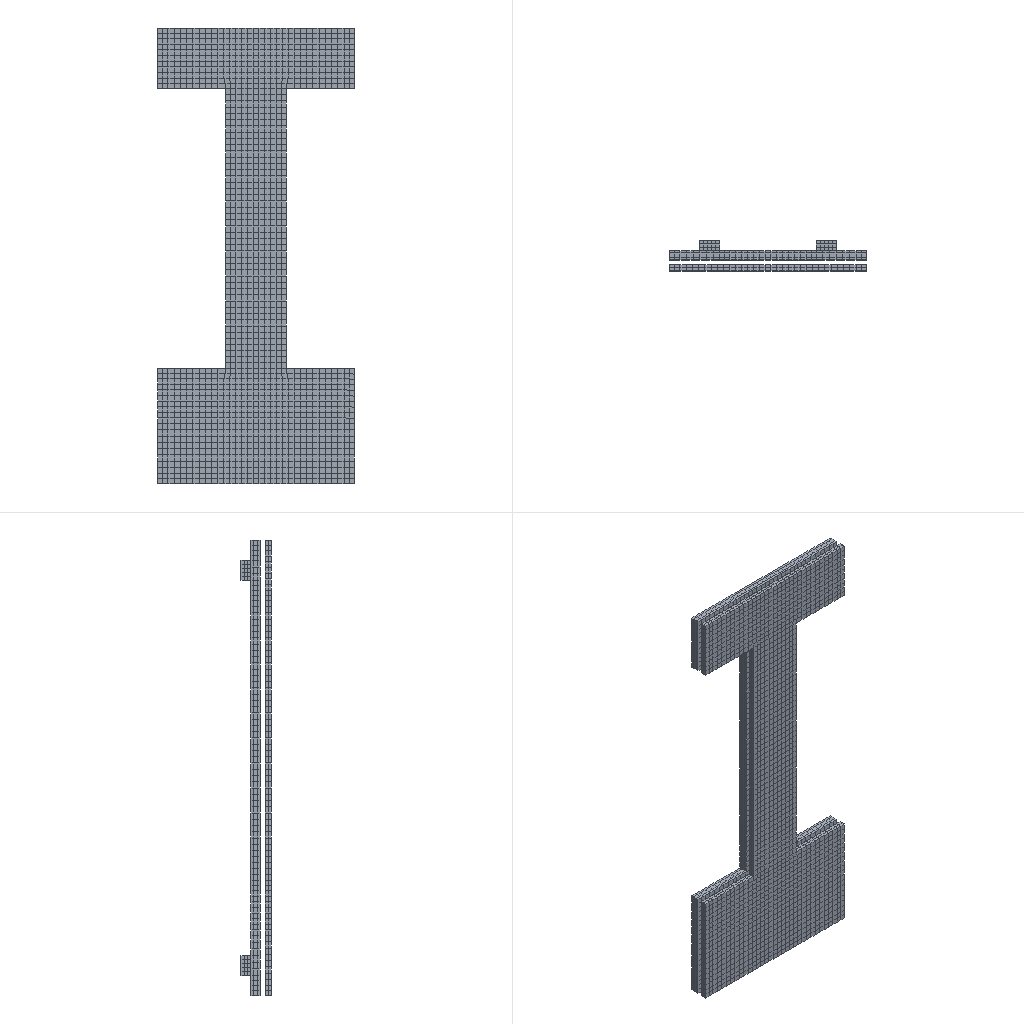Simulation study | abaqus
Set-up summary:
category,name,step,type,value,unit,region
solver,abaqus
solver,version,,,Abaqus/Standard 2020
units,not stated in the deck,,not stated
analysis,deck,,static,static
load_step,Step-1,Step-1,static
load_step,requested,,,1
mesh,nodes,,,12262
mesh,elements,,,7992
element_type,B31,,beam,102
element_type,C3D8R,,solid,7890
load,load commands in deck,,count,1
bc,support commands in deck,,count,2
material,C40P,,in results
material,CDP_C40(SEELEBIHAN),,in results
material,FRP,,in results
material,HRB400,,in results
material,SI_MM111111_Q235,,in results
material,SI_MM111111_Q345,,in results
check,setup vs results,,match,"per instance, exact: element labels, types and connectivity; labels of the nodes the elements use; coordinates of those nodes at SINGLE_PRECISION in 16 of 40 instance(s)"
Abaqus input file, long lists of numbers shortened:
*Heading
** Job name: Job-1 Model name: T1
** Generated by: Abaqus/CAE 2020
*Preprint, echo=NO, model=NO, history=NO, contact=NO
**
** PARTS
**
*Part, name=BetonAussen
*Node
      1,        -360.,       -1250.,          30.
      2,        -360.,       -1250.,           0.
** (4948 more lines like these left out)
*Element, type=C3D8R
 1,  285,  293, 2045, 1996,    1,    2,  244,  257
 2, 1996, 2045, 2046, 1997,  257,  244,  245,  256
** (3034 more lines like these left out)
*Nset, nset=Set-1, generate
    1,  4950,     1
*Elset, elset=Set-1, generate
    1,  3036,     1
** Section: Beton
*Solid Section, elset=Set-1, material=C40P
,
*End Part
**
*Part, name=BetonInnen
*Node
      1,         220.,        -400.,           0.
      2,         220.,        -400.,          24.
** (6598 more lines like these left out)
*Element, type=C3D8R
 1,  670,  678, 3475, 3433,    1,    2,  633,  644
 2, 3433, 3475, 3476, 3434,  644,  633,  634,  643
** (4552 more lines like these left out)
*Nset, nset=Set-1, generate
    1,  6600,     1
*Elset, elset=Set-1, generate
    1,  4554,     1
** Section: Beton
*Solid Section, elset=Set-1, material=C40P
,
*End Part
**
*Part, name=FRP
*Node
      1,         -35.,           0.,           0.
      2,          -5.,           0.,           0.
** (2 more lines like these left out)
*Element, type=B31
1, 2, 1
2, 2, 3
** (1 more lines like these left out)
*Nset, nset=Set-2, generate
 1,  4,  1
*Elset, elset=Set-2, generate
 1,  3,  1
*Nset, nset=Set-3, generate
 1,  4,  1
*Elset, elset=Set-3, generate
 1,  3,  1
*Nset, nset=Set-4, generate
 1,  4,  1
*Elset, elset=Set-4, generate
 1,  3,  1
** Section: FRP  Profile: Profile-1
*Beam Section, elset=Set-2, material=FRP, temperature=GRADIENTS, section=RECT
7., 7.
0.,0.,-1.
*End Part
**
*Part, name=Stuzen
*Node
      1,         -70.,        -52.5,         100.
      2,         -70.,        -12.5,         100.
** (142 more lines like these left out)
*Element, type=C3D8R
 1,  25,  26,  32,  31,   1,   2,   8,   7
 2,  26,  27,  33,  32,   2,   3,   9,   8
** (73 more lines like these left out)
*Nset, nset=Set-1, generate
   1,  144,    1
*Elset, elset=Set-1, generate
  1,  75,   1
** Section: Stutzen
*Solid Section, elset=Set-1, material=SI_mm111111_Q345
,
*End Part
**
**
** ASSEMBLY
**
*Assembly, name=Assembly
**
*Instance, name=BetonAussen-1, part=BetonAussen
        960.,          60.,       -2700.
        960.,          60.,       -2700., 961.,          60.,       -2700., 90.
*End Instance
**
*Instance, name=BetonInnen-1, part=BetonInnen
        960.,         200.,       -2700.
        960.,         200.,       -2700., 961.,         200.,       -2700., 90.
*End Instance
**
*Instance, name=Stuzen-1, part=Stuzen
       1530.,         200.,       -252.5
       1530.,         200.,       -252.5, 1529.,         200.,       -252.5, 90.
*End Instance
**
*Instance, name=Stuzen-1-lin-2-1, part=Stuzen
        370.,         200.,       -252.5
        370.,         200.,       -252.5, 369.,         200.,       -252.5, 90.
*End Instance
**
*Instance, name=Stuzen-1-lin-3-1, part=Stuzen
       1530.,         200.,      -4202.5
       1530.,         200.,      -4202.5, 1529.,         200.,      -4202.5, 90.
*End Instance
**
*Instance, name=Stuzen-1-lin-4-1, part=Stuzen
        370.,         200.,      -4202.5
        370.,         200.,      -4202.5, 369.,         200.,      -4202.5, 90.
*End Instance
**
*Instance, name=FRP-1, part=FRP
       1860.,          65.,        -100.
       1860.,          65.,        -100.,        1860.,          65., -99., 90.
*End Instance
**
*Instance, name=FRP-1-lin-2-1, part=FRP
       1860.,          65.,        -500.
       1860.,          65.,        -500.,        1860.,          65., -499., 90.
*End Instance
**
*Instance, name=FRP-1-lin-3-1, part=FRP
       1360.,          65.,        -100.
       1360.,          65.,        -100.,        1360.,          65., -99., 90.
*End Instance
**
*Instance, name=FRP-1-lin-4-1, part=FRP
       1360.,          65.,        -500.
       1360.,          65.,        -500.,        1360.,          65., -499., 90.
*End Instance
**
*Instance, name=FRP-1-lin-5-1, part=FRP
        600.,          65.,        -100.
        600.,          65.,        -100.,         600.,          65., -99., 90.
*End Instance
**
*Instance, name=FRP-1-lin-6-1, part=FRP
        600.,          65.,        -500.
        600.,          65.,        -500.,         600.,          65., -499., 90.
*End Instance
**
*Instance, name=FRP-1-lin-7-1, part=FRP
        100.,          65.,        -100.
        100.,          65.,        -100.,         100.,          65., -99., 90.
*End Instance
**
*Instance, name=FRP-1-lin-8-1, part=FRP
        100.,          65.,        -500.
        100.,          65.,        -500.,         100.,          65., -499., 90.
*End Instance
**
*Instance, name=FRP-1-lin-9-1, part=FRP
       1180.,          65.,       -1100.
       1180.,          65.,       -1100.,        1180.,          65., -1099., 90.
*End Instance
**
*Instance, name=FRP-1-lin-10-1, part=FRP
       1180.,          65.,        -600.
       1180.,          65.,        -600.,        1180.,          65., -599., 90.
*End Instance
**
*Instance, name=FRP-1-lin-11-1, part=FRP
        780.,          65.,        -600.
        780.,          65.,        -600.,         780.,          65., -599., 90.
*End Instance
**
*Instance, name=FRP-1-lin-12-1, part=FRP
        780.,          65.,       -1100.
        780.,          65.,       -1100.,         780.,          65., -1099., 90.
*End Instance
**
*Instance, name=FRP-1-lin-9-1-lin-1-2, part=FRP
       1180.,          65.,       -1600.
       1180.,          65.,       -1600.,        1180.,          65., -1599., 90.
*End Instance
**
*Instance, name=FRP-1-lin-9-1-lin-1-3, part=FRP
       1180.,          65.,       -2100.
       1180.,          65.,       -2100.,        1180.,          65., -2099., 90.
*End Instance
**
*Instance, name=FRP-1-lin-9-1-lin-1-4, part=FRP
       1180.,          65.,       -2600.
       1180.,          65.,       -2600.,        1180.,          65., -2599., 90.
*End Instance
**
*Instance, name=FRP-1-lin-9-1-lin-1-5, part=FRP
       1180.,          65.,       -3100.
       1180.,          65.,       -3100.,        1180.,          65., -3099., 90.
*End Instance
**
*Instance, name=FRP-1-lin-12-1-lin-1-2, part=FRP
        780.,          65.,       -1600.
        780.,          65.,       -1600.,         780.,          65., -1599., 90.
*End Instance
**
*Instance, name=FRP-1-lin-12-1-lin-1-3, part=FRP
        780.,          65.,       -2100.
        780.,          65.,       -2100.,         780.,          65., -2099., 90.
*End Instance
**
*Instance, name=FRP-1-lin-12-1-lin-1-4, part=FRP
        780.,          65.,       -2600.
        780.,          65.,       -2600.,         780.,          65., -2599., 90.
*End Instance
**
*Instance, name=FRP-1-lin-12-1-lin-1-5, part=FRP
        780.,          65.,       -3100.
        780.,          65.,       -3100.,         780.,          65., -3099., 90.
*End Instance
**
*Instance, name=FRP-1-lin-12-1-lin-1-6, part=FRP
        780.,          65.,       -3400.
        780.,          65.,       -3400.,         780.,          65., -3399., 90.
*End Instance
**
*Instance, name=FRP-1-lin-9-1-lin-1-6-lin-1-2, part=FRP
       1860.,          65.,       -3520.
       1860.,          65.,       -3520.,        1860.,          65., -3519., 90.
*End Instance
**
*Instance, name=FRP-1-lin-9-1-lin-1-6-lin-1-3, part=FRP
       1360.,          65.,       -3950.
       1360.,          65.,       -3950.,        1360.,          65., -3949., 90.
*End Instance
**
*Instance, name=FRP-1-lin-9-1-lin-1-6-lin-1-4, part=FRP
       1360.,          65.,       -4450.
       1360.,          65.,       -4450.,        1360.,          65., -4449., 90.
*End Instance
**
*Instance, name=FRP-1-lin-9-1-lin-1-6-lin-1-5, part=FRP
        600.,          65.,       -3500.
        600.,          65.,       -3500.,         600.,          65., -3499., 90.
*End Instance
**
*Instance, name=FRP-1-lin-9-1-lin-1-6-lin-1-6, part=FRP
        100.,          65.,       -4450.
        100.,          65.,       -4450.,         100.,          65., -4449., 90.
*End Instance
**
*Instance, name=FRP-1-lin-9-1-lin-1-6-lin-1-7, part=FRP
        100.,          65.,       -3500.
        100.,          65.,       -3500.,         100.,          65., -3499., 90.
*End Instance
**
*Instance, name=FRP-1-lin-9-1-lin-1-6-lin-2-1, part=FRP
       1180.,          65.,       -3400.
       1180.,          65.,       -3400.,        1180.,          65., -3399., 90.
*End Instance
**
*Instance, name=FRP-1-lin-9-1-lin-1-6-lin-2-2, part=FRP
       1360.,          65.,       -3500.
       1360.,          65.,       -3500.,        1360.,          65., -3499., 90.
*End Instance
**
*Instance, name=FRP-1-lin-9-1-lin-1-6-lin-2-3, part=FRP
       1860.,          65.,       -3950.
       1860.,          65.,       -3950.,        1860.,          65., -3949., 90.
*End Instance
**
*Instance, name=FRP-1-lin-9-1-lin-1-6-lin-2-4, part=FRP
       1860.,          65.,       -4450.
       1860.,          65.,       -4450.,        1860.,          65., -4449., 90.
*End Instance
**
*Instance, name=FRP-1-lin-9-1-lin-1-6-lin-2-5, part=FRP
        600.,          65.,       -3950.
        600.,          65.,       -3950.,         600.,          65., -3949., 90.
*End Instance
**
*Instance, name=FRP-1-lin-9-1-lin-1-6-lin-2-6, part=FRP
        600.,          65.,       -4450.
        600.,          65.,       -4450.,         600.,          65., -4449., 90.
*End Instance
**
*Instance, name=FRP-1-lin-9-1-lin-1-6-lin-2-5-lin-1-2, part=FRP
        100.,          65.,       -3950.
        100.,          65.,       -3950.,         100.,          65., -3949., 90.
*End Instance
**
*Node
      1,        1560.,         300.,        -300.
*Node
      2,         400.,         300.,        -300.
*Node
      3,        1560.,         300.,       -4250.
*Node
      4,         400.,         300.,       -4250.
*Nset, nset=BetonAussen, instance=BetonAussen-1, generate
    1,  4950,     1
*Elset, elset=BetonAussen, instance=BetonAussen-1, generate
    1,  3036,     1
*Nset, nset=BetonInnen, instance=BetonInnen-1, generate
    1,  6600,     1
*Elset, elset=BetonInnen, instance=BetonInnen-1, generate
    1,  4554,     1
*Nset, nset=NZAussen, instance=FRP-1
 1, 2
*Nset, nset=NZAussen, instance=FRP-1-lin-2-1
 1, 2
*Nset, nset=NZAussen, instance=FRP-1-lin-3-1
 1, 2
*Nset, nset=NZAussen, instance=FRP-1-lin-7-1
 1, 2
*Nset, nset=NZAussen, instance=FRP-1-lin-11-1
 1, 2
*Nset, nset=NZAussen, instance=FRP-1-lin-12-1-lin-1-2
 1, 2
*Nset, nset=NZAussen, instance=FRP-1-lin-9-1-lin-1-6-lin-2-3
 1, 2
*Nset, nset=NZAussen, instance=FRP-1-lin-9-1-lin-1-6-lin-1-5
 1, 2
*Nset, nset=NZAussen, instance=FRP-1-lin-9-1-lin-1-3
 1, 2
*Nset, nset=NZAussen, instance=FRP-1-lin-12-1-lin-1-6
 1, 2
*Nset, nset=NZAussen, instance=FRP-1-lin-9-1-lin-1-6-lin-2-5-lin-1-2
 1, 2
*Nset, nset=NZAussen, instance=FRP-1-lin-5-1
 1, 2
*Nset, nset=NZAussen, instance=FRP-1-lin-12-1-lin-1-4
 1, 2
*Nset, nset=NZAussen, instance=FRP-1-lin-9-1-lin-1-6-lin-2-5
 1, 2
*Nset, nset=NZAussen, instance=FRP-1-lin-9-1-lin-1-6-lin-1-7
 1, 2
*Nset, nset=NZAussen, instance=FRP-1-lin-9-1
 1, 2
*Nset, nset=NZAussen, instance=FRP-1-lin-9-1-lin-1-6-lin-1-3
 1, 2
*Nset, nset=NZAussen, instance=FRP-1-lin-9-1-lin-1-5
 1, 2
*Nset, nset=NZAussen, instance=FRP-1-lin-9-1-lin-1-6-lin-2-1
 1, 2
*Nset, nset=NZAussen, instance=FRP-1-lin-4-1
 1, 2
*Nset, nset=NZAussen, instance=FRP-1-lin-8-1
 1, 2
*Nset, nset=NZAussen, instance=FRP-1-lin-12-1
 1, 2
*Nset, nset=NZAussen, instance=FRP-1-lin-12-1-lin-1-3
 1, 2
*Nset, nset=NZAussen, instance=FRP-1-lin-9-1-lin-1-6-lin-2-4
 1, 2
*Nset, nset=NZAussen, instance=FRP-1-lin-9-1-lin-1-6-lin-1-6
 1, 2
*Nset, nset=NZAussen, instance=FRP-1-lin-9-1-lin-1-4
 1, 2
*Nset, nset=NZAussen, instance=FRP-1-lin-9-1-lin-1-6-lin-1-2
 1, 2
*Nset, nset=NZAussen, instance=FRP-1-lin-6-1
 1, 2
*Nset, nset=NZAussen, instance=FRP-1-lin-9-1-lin-1-2
 1, 2
*Nset, nset=NZAussen, instance=FRP-1-lin-12-1-lin-1-5
 1, 2
*Nset, nset=NZAussen, instance=FRP-1-lin-9-1-lin-1-6-lin-2-6
 1, 2
*Nset, nset=NZAussen, instance=FRP-1-lin-10-1
 1, 2
*Nset, nset=NZAussen, instance=FRP-1-lin-9-1-lin-1-6-lin-1-4
 1, 2
*Nset, nset=NZAussen, instance=FRP-1-lin-9-1-lin-1-6-lin-2-2
 1, 2
*Elset, elset=NZAussen, instance=FRP-1
 1,
*Elset, elset=NZAussen, instance=FRP-1-lin-2-1
 1,
*Elset, elset=NZAussen, instance=FRP-1-lin-3-1
 1,
*Elset, elset=NZAussen, instance=FRP-1-lin-7-1
 1,
*Elset, elset=NZAussen, instance=FRP-1-lin-11-1
 1,
*Elset, elset=NZAussen, instance=FRP-1-lin-12-1-lin-1-2
 1,
*Elset, elset=NZAussen, instance=FRP-1-lin-9-1-lin-1-6-lin-2-3
 1,
*Elset, elset=NZAussen, instance=FRP-1-lin-9-1-lin-1-6-lin-1-5
 1,
*Elset, elset=NZAussen, instance=FRP-1-lin-9-1-lin-1-3
 1,
*Elset, elset=NZAussen, instance=FRP-1-lin-12-1-lin-1-6
 1,
*Elset, elset=NZAussen, instance=FRP-1-lin-9-1-lin-1-6-lin-2-5-lin-1-2
 1,
*Elset, elset=NZAussen, instance=FRP-1-lin-5-1
 1,
*Elset, elset=NZAussen, instance=FRP-1-lin-12-1-lin-1-4
 1,
*Elset, elset=NZAussen, instance=FRP-1-lin-9-1-lin-1-6-lin-2-5
 1,
*Elset, elset=NZAussen, instance=FRP-1-lin-9-1-lin-1-6-lin-1-7
 1,
*Elset, elset=NZAussen, instance=FRP-1-lin-9-1
 1,
*Elset, elset=NZAussen, instance=FRP-1-lin-9-1-lin-1-6-lin-1-3
 1,
*Elset, elset=NZAussen, instance=FRP-1-lin-9-1-lin-1-5
 1,
*Elset, elset=NZAussen, instance=FRP-1-lin-9-1-lin-1-6-lin-2-1
 1,
*Elset, elset=NZAussen, instance=FRP-1-lin-4-1
 1,
*Elset, elset=NZAussen, instance=FRP-1-lin-8-1
 1,
*Elset, elset=NZAussen, instance=FRP-1-lin-12-1
 1,
*Elset, elset=NZAussen, instance=FRP-1-lin-12-1-lin-1-3
 1,
*Elset, elset=NZAussen, instance=FRP-1-lin-9-1-lin-1-6-lin-2-4
 1,
*Elset, elset=NZAussen, instance=FRP-1-lin-9-1-lin-1-6-lin-1-6
 1,
*Elset, elset=NZAussen, instance=FRP-1-lin-9-1-lin-1-4
 1,
*Elset, elset=NZAussen, instance=FRP-1-lin-9-1-lin-1-6-lin-1-2
 1,
*Elset, elset=NZAussen, instance=FRP-1-lin-6-1
 1,
*Elset, elset=NZAussen, instance=FRP-1-lin-9-1-lin-1-2
 1,
*Elset, elset=NZAussen, instance=FRP-1-lin-12-1-lin-1-5
 1,
*Elset, elset=NZAussen, instance=FRP-1-lin-9-1-lin-1-6-lin-2-6
 1,
*Elset, elset=NZAussen, instance=FRP-1-lin-10-1
 1,
*Elset, elset=NZAussen, instance=FRP-1-lin-9-1-lin-1-6-lin-1-4
 1,
*Elset, elset=NZAussen, instance=FRP-1-lin-9-1-lin-1-6-lin-2-2
 1,
*Nset, nset=NZInnen, instance=FRP-1
 3, 4
*Nset, nset=NZInnen, instance=FRP-1-lin-2-1
 3, 4
*Nset, nset=NZInnen, instance=FRP-1-lin-3-1
 3, 4
*Nset, nset=NZInnen, instance=FRP-1-lin-7-1
 3, 4
*Nset, nset=NZInnen, instance=FRP-1-lin-11-1
 3, 4
*Nset, nset=NZInnen, instance=FRP-1-lin-12-1-lin-1-2
 3, 4
*Nset, nset=NZInnen, instance=FRP-1-lin-9-1-lin-1-6-lin-2-3
 3, 4
*Nset, nset=NZInnen, instance=FRP-1-lin-9-1-lin-1-6-lin-1-5
 3, 4
*Nset, nset=NZInnen, instance=FRP-1-lin-9-1-lin-1-3
 3, 4
*Nset, nset=NZInnen, instance=FRP-1-lin-12-1-lin-1-6
 3, 4
*Nset, nset=NZInnen, instance=FRP-1-lin-9-1-lin-1-6-lin-2-5-lin-1-2
 3, 4
*Nset, nset=NZInnen, instance=FRP-1-lin-5-1
 3, 4
*Nset, nset=NZInnen, instance=FRP-1-lin-12-1-lin-1-4
 3, 4
*Nset, nset=NZInnen, instance=FRP-1-lin-9-1-lin-1-6-lin-2-5
 3, 4
*Nset, nset=NZInnen, instance=FRP-1-lin-9-1-lin-1-6-lin-1-7
 3, 4
*Nset, nset=NZInnen, instance=FRP-1-lin-9-1
 3, 4
*Nset, nset=NZInnen, instance=FRP-1-lin-9-1-lin-1-6-lin-1-3
 3, 4
*Nset, nset=NZInnen, instance=FRP-1-lin-9-1-lin-1-5
 3, 4
*Nset, nset=NZInnen, instance=FRP-1-lin-9-1-lin-1-6-lin-2-1
 3, 4
*Nset, nset=NZInnen, instance=FRP-1-lin-4-1
 3, 4
*Nset, nset=NZInnen, instance=FRP-1-lin-8-1
 3, 4
*Nset, nset=NZInnen, instance=FRP-1-lin-12-1
 3, 4
*Nset, nset=NZInnen, instance=FRP-1-lin-12-1-lin-1-3
 3, 4
*Nset, nset=NZInnen, instance=FRP-1-lin-9-1-lin-1-6-lin-2-4
 3, 4
*Nset, nset=NZInnen, instance=FRP-1-lin-9-1-lin-1-6-lin-1-6
 3, 4
*Nset, nset=NZInnen, instance=FRP-1-lin-9-1-lin-1-4
 3, 4
*Nset, nset=NZInnen, instance=FRP-1-lin-9-1-lin-1-6-lin-1-2
 3, 4
*Nset, nset=NZInnen, instance=FRP-1-lin-6-1
 3, 4
*Nset, nset=NZInnen, instance=FRP-1-lin-9-1-lin-1-2
 3, 4
*Nset, nset=NZInnen, instance=FRP-1-lin-12-1-lin-1-5
 3, 4
*Nset, nset=NZInnen, instance=FRP-1-lin-9-1-lin-1-6-lin-2-6
 3, 4
*Nset, nset=NZInnen, instance=FRP-1-lin-10-1
 3, 4
*Nset, nset=NZInnen, instance=FRP-1-lin-9-1-lin-1-6-lin-1-4
 3, 4
*Nset, nset=NZInnen, instance=FRP-1-lin-9-1-lin-1-6-lin-2-2
 3, 4
*Elset, elset=NZInnen, instance=FRP-1
 3,
*Elset, elset=NZInnen, instance=FRP-1-lin-2-1
 3,
*Elset, elset=NZInnen, instance=FRP-1-lin-3-1
 3,
*Elset, elset=NZInnen, instance=FRP-1-lin-7-1
 3,
*Elset, elset=NZInnen, instance=FRP-1-lin-11-1
 3,
*Elset, elset=NZInnen, instance=FRP-1-lin-12-1-lin-1-2
 3,
*Elset, elset=NZInnen, instance=FRP-1-lin-9-1-lin-1-6-lin-2-3
 3,
*Elset, elset=NZInnen, instance=FRP-1-lin-9-1-lin-1-6-lin-1-5
 3,
*Elset, elset=NZInnen, instance=FRP-1-lin-9-1-lin-1-3
 3,
*Elset, elset=NZInnen, instance=FRP-1-lin-12-1-lin-1-6
 3,
*Elset, elset=NZInnen, instance=FRP-1-lin-9-1-lin-1-6-lin-2-5-lin-1-2
 3,
*Elset, elset=NZInnen, instance=FRP-1-lin-5-1
 3,
*Elset, elset=NZInnen, instance=FRP-1-lin-12-1-lin-1-4
 3,
*Elset, elset=NZInnen, instance=FRP-1-lin-9-1-lin-1-6-lin-2-5
 3,
*Elset, elset=NZInnen, instance=FRP-1-lin-9-1-lin-1-6-lin-1-7
 3,
*Elset, elset=NZInnen, instance=FRP-1-lin-9-1
 3,
*Elset, elset=NZInnen, instance=FRP-1-lin-9-1-lin-1-6-lin-1-3
 3,
*Elset, elset=NZInnen, instance=FRP-1-lin-9-1-lin-1-5
 3,
*Elset, elset=NZInnen, instance=FRP-1-lin-9-1-lin-1-6-lin-2-1
 3,
*Elset, elset=NZInnen, instance=FRP-1-lin-4-1
 3,
*Elset, elset=NZInnen, instance=FRP-1-lin-8-1
 3,
*Elset, elset=NZInnen, instance=FRP-1-lin-12-1
 3,
*Elset, elset=NZInnen, instance=FRP-1-lin-12-1-lin-1-3
 3,
*Elset, elset=NZInnen, instance=FRP-1-lin-9-1-lin-1-6-lin-2-4
 3,
*Elset, elset=NZInnen, instance=FRP-1-lin-9-1-lin-1-6-lin-1-6
 3,
*Elset, elset=NZInnen, instance=FRP-1-lin-9-1-lin-1-4
 3,
*Elset, elset=NZInnen, instance=FRP-1-lin-9-1-lin-1-6-lin-1-2
 3,
*Elset, elset=NZInnen, instance=FRP-1-lin-6-1
 3,
*Elset, elset=NZInnen, instance=FRP-1-lin-9-1-lin-1-2
 3,
*Elset, elset=NZInnen, instance=FRP-1-lin-12-1-lin-1-5
 3,
*Elset, elset=NZInnen, instance=FRP-1-lin-9-1-lin-1-6-lin-2-6
 3,
*Elset, elset=NZInnen, instance=FRP-1-lin-10-1
 3,
*Elset, elset=NZInnen, instance=FRP-1-lin-9-1-lin-1-6-lin-1-4
 3,
*Elset, elset=NZInnen, instance=FRP-1-lin-9-1-lin-1-6-lin-2-2
 3,
*Nset, nset=RFP, instance=FRP-1, generate
 1,  4,  1
*Nset, nset=RFP, generate
 1,  4,  1
*Nset, nset=RFP, instance=FRP-1-lin-2-1, generate
 1,  4,  1
*Nset, nset=RFP, instance=FRP-1-lin-3-1, generate
 1,  4,  1
*Nset, nset=RFP, instance=FRP-1-lin-7-1, generate
 1,  4,  1
*Nset, nset=RFP, instance=FRP-1-lin-11-1, generate
 1,  4,  1
*Nset, nset=RFP, instance=FRP-1-lin-12-1-lin-1-2, generate
 1,  4,  1
*Nset, nset=RFP, instance=FRP-1-lin-9-1-lin-1-6-lin-2-3, generate
 1,  4,  1
*Nset, nset=RFP, instance=FRP-1-lin-9-1-lin-1-6-lin-1-5, generate
 1,  4,  1
*Nset, nset=RFP, instance=FRP-1-lin-9-1-lin-1-3, generate
 1,  4,  1
*Nset, nset=RFP, instance=FRP-1-lin-12-1-lin-1-6, generate
 1,  4,  1
*Nset, nset=RFP, instance=FRP-1-lin-9-1-lin-1-6-lin-2-5-lin-1-2, generate
 1,  4,  1
*Nset, nset=RFP, instance=FRP-1-lin-5-1, generate
 1,  4,  1
*Nset, nset=RFP, instance=FRP-1-lin-12-1-lin-1-4, generate
 1,  4,  1
*Nset, nset=RFP, instance=FRP-1-lin-9-1-lin-1-6-lin-2-5, generate
 1,  4,  1
*Nset, nset=RFP, instance=FRP-1-lin-9-1-lin-1-6-lin-1-7, generate
 1,  4,  1
*Nset, nset=RFP, instance=FRP-1-lin-9-1, generate
 1,  4,  1
*Nset, nset=RFP, instance=FRP-1-lin-9-1-lin-1-6-lin-1-3, generate
 1,  4,  1
*Nset, nset=RFP, instance=FRP-1-lin-9-1-lin-1-5, generate
 1,  4,  1
*Nset, nset=RFP, instance=FRP-1-lin-9-1-lin-1-6-lin-2-1, generate
 1,  4,  1
*Nset, nset=RFP, instance=FRP-1-lin-4-1, generate
 1,  4,  1
*Nset, nset=RFP, instance=FRP-1-lin-8-1, generate
 1,  4,  1
*Nset, nset=RFP, instance=FRP-1-lin-12-1, generate
 1,  4,  1
*Nset, nset=RFP, instance=FRP-1-lin-12-1-lin-1-3, generate
 1,  4,  1
*Nset, nset=RFP, instance=FRP-1-lin-9-1-lin-1-6-lin-2-4, generate
 1,  4,  1
*Nset, nset=RFP, instance=FRP-1-lin-9-1-lin-1-6-lin-1-6, generate
 1,  4,  1
*Nset, nset=RFP, instance=FRP-1-lin-9-1-lin-1-4, generate
 1,  4,  1
*Nset, nset=RFP, instance=FRP-1-lin-9-1-lin-1-6-lin-1-2, generate
 1,  4,  1
*Nset, nset=RFP, instance=FRP-1-lin-6-1, generate
 1,  4,  1
*Nset, nset=RFP, instance=FRP-1-lin-9-1-lin-1-2, generate
 1,  4,  1
*Nset, nset=RFP, instance=FRP-1-lin-12-1-lin-1-5, generate
 1,  4,  1
*Nset, nset=RFP, instance=FRP-1-lin-9-1-lin-1-6-lin-2-6, generate
 1,  4,  1
*Nset, nset=RFP, instance=FRP-1-lin-10-1, generate
 1,  4,  1
*Nset, nset=RFP, instance=FRP-1-lin-9-1-lin-1-6-lin-1-4, generate
 1,  4,  1
*Nset, nset=RFP, instance=FRP-1-lin-9-1-lin-1-6-lin-2-2, generate
 1,  4,  1
*Elset, elset=RFP, instance=FRP-1, generate
 1,  3,  1
*Elset, elset=RFP, instance=FRP-1-lin-2-1, generate
 1,  3,  1
*Elset, elset=RFP, instance=FRP-1-lin-3-1, generate
 1,  3,  1
*Elset, elset=RFP, instance=FRP-1-lin-7-1, generate
 1,  3,  1
*Elset, elset=RFP, instance=FRP-1-lin-11-1, generate
 1,  3,  1
*Elset, elset=RFP, instance=FRP-1-lin-12-1-lin-1-2, generate
 1,  3,  1
*Elset, elset=RFP, instance=FRP-1-lin-9-1-lin-1-6-lin-2-3, generate
 1,  3,  1
*Elset, elset=RFP, instance=FRP-1-lin-9-1-lin-1-6-lin-1-5, generate
 1,  3,  1
*Elset, elset=RFP, instance=FRP-1-lin-9-1-lin-1-3, generate
 1,  3,  1
*Elset, elset=RFP, instance=FRP-1-lin-12-1-lin-1-6, generate
 1,  3,  1
*Elset, elset=RFP, instance=FRP-1-lin-9-1-lin-1-6-lin-2-5-lin-1-2, generate
 1,  3,  1
*Elset, elset=RFP, instance=FRP-1-lin-5-1, generate
 1,  3,  1
*Elset, elset=RFP, instance=FRP-1-lin-12-1-lin-1-4, generate
 1,  3,  1
*Elset, elset=RFP, instance=FRP-1-lin-9-1-lin-1-6-lin-2-5, generate
 1,  3,  1
*Elset, elset=RFP, instance=FRP-1-lin-9-1-lin-1-6-lin-1-7, generate
 1,  3,  1
*Elset, elset=RFP, instance=FRP-1-lin-9-1, generate
 1,  3,  1
*Elset, elset=RFP, instance=FRP-1-lin-9-1-lin-1-6-lin-1-3, generate
 1,  3,  1
*Elset, elset=RFP, instance=FRP-1-lin-9-1-lin-1-5, generate
 1,  3,  1
*Elset, elset=RFP, instance=FRP-1-lin-9-1-lin-1-6-lin-2-1, generate
 1,  3,  1
*Elset, elset=RFP, instance=FRP-1-lin-4-1, generate
 1,  3,  1
*Elset, elset=RFP, instance=FRP-1-lin-8-1, generate
 1,  3,  1
*Elset, elset=RFP, instance=FRP-1-lin-12-1, generate
 1,  3,  1
*Elset, elset=RFP, instance=FRP-1-lin-12-1-lin-1-3, generate
 1,  3,  1
*Elset, elset=RFP, instance=FRP-1-lin-9-1-lin-1-6-lin-2-4, generate
 1,  3,  1
*Elset, elset=RFP, instance=FRP-1-lin-9-1-lin-1-6-lin-1-6, generate
 1,  3,  1
*Elset, elset=RFP, instance=FRP-1-lin-9-1-lin-1-4, generate
 1,  3,  1
*Elset, elset=RFP, instance=FRP-1-lin-9-1-lin-1-6-lin-1-2, generate
 1,  3,  1
*Elset, elset=RFP, instance=FRP-1-lin-6-1, generate
 1,  3,  1
*Elset, elset=RFP, instance=FRP-1-lin-9-1-lin-1-2, generate
 1,  3,  1
*Elset, elset=RFP, instance=FRP-1-lin-12-1-lin-1-5, generate
 1,  3,  1
*Elset, elset=RFP, instance=FRP-1-lin-9-1-lin-1-6-lin-2-6, generate
 1,  3,  1
*Elset, elset=RFP, instance=FRP-1-lin-10-1, generate
 1,  3,  1
*Elset, elset=RFP, instance=FRP-1-lin-9-1-lin-1-6-lin-1-4, generate
 1,  3,  1
*Elset, elset=RFP, instance=FRP-1-lin-9-1-lin-1-6-lin-2-2, generate
 1,  3,  1
*Nset, nset=Set-19
 1, 2
*Nset, nset=Set-20
 3, 4
*Elset, elset=Set-down, instance=FRP-1-lin-9-1-lin-1-6-lin-1-2
 1,
*Elset, elset=Set-down, instance=FRP-1-lin-9-1-lin-1-6-lin-1-3
 1,
*Elset, elset=Set-down, instance=FRP-1-lin-9-1-lin-1-6-lin-1-5
 1,
*Elset, elset=Set-down, instance=FRP-1-lin-9-1-lin-1-6-lin-2-3
 1,
*Elset, elset=Set-down, instance=FRP-1-lin-12-1-lin-1-2
 1,
*Elset, elset=Set-down, instance=FRP-1-lin-3-1
 1,
*Elset, elset=Set-down, instance=FRP-1-lin-11-1
 1,
*Elset, elset=Set-down, instance=FRP-1-lin-9-1-lin-1-6-lin-2-5-lin-1-2
 1,
*Elset, elset=Set-down, instance=FRP-1-lin-12-1-lin-1-6
 1,
*Elset, elset=Set-down, instance=FRP-1-lin-7-1
 1,
*Elset, elset=Set-down, instance=FRP-1-lin-9-1-lin-1-3
 1,
*Elset, elset=Set-down, instance=FRP-1-lin-9-1-lin-1-6-lin-1-7
 1,
*Elset, elset=Set-down, instance=FRP-1-lin-9-1-lin-1-6-lin-2-5
 1,
*Elset, elset=Set-down, instance=FRP-1-lin-12-1-lin-1-4
 1,
*Elset, elset=Set-down, instance=FRP-1-lin-5-1
 1,
*Elset, elset=Set-down, instance=FRP-1
 1,
*Elset, elset=Set-down, instance=FRP-1-lin-9-1-lin-1-6-lin-2-1
 1,
*Elset, elset=Set-down, instance=FRP-1-lin-9-1
 1,
*Elset, elset=Set-down, instance=FRP-1-lin-9-1-lin-1-5
 1,
*Elset, elset=Set-down, instance=FRP-1-lin-9-1-lin-1-6-lin-1-4
 1,
*Elset, elset=Set-down, instance=FRP-1-lin-9-1-lin-1-6-lin-1-6
 1,
*Elset, elset=Set-down, instance=FRP-1-lin-9-1-lin-1-6-lin-2-4
 1,
*Elset, elset=Set-down, instance=FRP-1-lin-12-1-lin-1-3
 1,
*Elset, elset=Set-down, instance=FRP-1-lin-4-1
 1,
*Elset, elset=Set-down, instance=FRP-1-lin-12-1
 1,
*Elset, elset=Set-down, instance=FRP-1-lin-9-1-lin-1-4
 1,
*Elset, elset=Set-down, instance=FRP-1-lin-8-1
 1,
*Elset, elset=Set-down, instance=FRP-1-lin-9-1-lin-1-6-lin-2-2
 1,
*Elset, elset=Set-down, instance=FRP-1-lin-9-1-lin-1-6-lin-2-6
 1,
*Elset, elset=Set-down, instance=FRP-1-lin-12-1-lin-1-5
 1,
*Elset, elset=Set-down, instance=FRP-1-lin-6-1
 1,
*Elset, elset=Set-down, instance=FRP-1-lin-9-1-lin-1-2
 1,
*Elset, elset=Set-down, instance=FRP-1-lin-2-1
 1,
*Elset, elset=Set-down, instance=FRP-1-lin-10-1
 1,
*Elset, elset=Set-up, instance=FRP-1-lin-9-1-lin-1-6-lin-1-3
 3,
*Elset, elset=Set-up, instance=FRP-1-lin-9-1-lin-1-6-lin-1-4
 3,
*Elset, elset=Set-up, instance=FRP-1-lin-9-1-lin-1-6-lin-2-3
 3,
*Elset, elset=Set-up, instance=FRP-1-lin-9-1-lin-1-6-lin-2-5-lin-1-2
 3,
*Elset, elset=Set-up, instance=FRP-1-lin-9-1-lin-1-6-lin-1-5
 3,
*Elset, elset=Set-up, instance=FRP-1-lin-12-1-lin-1-2
 3,
*Elset, elset=Set-up, instance=FRP-1-lin-3-1
 3,
*Elset, elset=Set-up, instance=FRP-1-lin-11-1
 3,
*Elset, elset=Set-up, instance=FRP-1-lin-12-1-lin-1-6
 3,
*Elset, elset=Set-up, instance=FRP-1-lin-7-1
 3,
*Elset, elset=Set-up, instance=FRP-1-lin-9-1-lin-1-3
 3,
*Elset, elset=Set-up, instance=FRP-1-lin-9-1-lin-1-6-lin-2-5
 3,
*Elset, elset=Set-up, instance=FRP-1-lin-9-1-lin-1-6-lin-1-7
 3,
*Elset, elset=Set-up, instance=FRP-1-lin-12-1-lin-1-4
 3,
*Elset, elset=Set-up, instance=FRP-1-lin-5-1
 3,
*Elset, elset=Set-up, instance=FRP-1
 3,
*Elset, elset=Set-up, instance=FRP-1-lin-9-1-lin-1-6-lin-2-1
 3,
*Elset, elset=Set-up, instance=FRP-1-lin-9-1
 3,
*Elset, elset=Set-up, instance=FRP-1-lin-9-1-lin-1-5
 3,
*Elset, elset=Set-up, instance=FRP-1-lin-9-1-lin-1-6-lin-1-6
 3,
*Elset, elset=Set-up, instance=FRP-1-lin-9-1-lin-1-6-lin-2-4
 3,
*Elset, elset=Set-up, instance=FRP-1-lin-12-1-lin-1-3
 3,
*Elset, elset=Set-up, instance=FRP-1-lin-4-1
 3,
*Elset, elset=Set-up, instance=FRP-1-lin-12-1
 3,
*Elset, elset=Set-up, instance=FRP-1-lin-9-1-lin-1-6-lin-1-2
 3,
*Elset, elset=Set-up, instance=FRP-1-lin-8-1
 3,
*Elset, elset=Set-up, instance=FRP-1-lin-9-1-lin-1-4
 3,
*Elset, elset=Set-up, instance=FRP-1-lin-9-1-lin-1-6-lin-2-6
 3,
*Elset, elset=Set-up, instance=FRP-1-lin-12-1-lin-1-5
 3,
*Elset, elset=Set-up, instance=FRP-1-lin-6-1
 3,
*Elset, elset=Set-up, instance=FRP-1-lin-9-1-lin-1-2
 3,
*Elset, elset=Set-up, instance=FRP-1-lin-9-1-lin-1-6-lin-2-2
 3,
*Elset, elset=Set-up, instance=FRP-1-lin-10-1
 3,
*Elset, elset=Set-up, instance=FRP-1-lin-2-1
 3,
*Nset, nset=Stutzen, instance=Stuzen-1, generate
   1,  144,    1
*Nset, nset=Stutzen, instance=Stuzen-1-lin-2-1, generate
   1,  144,    1
*Nset, nset=Stutzen, instance=Stuzen-1-lin-3-1, generate
   1,  144,    1
*Nset, nset=Stutzen, instance=Stuzen-1-lin-4-1, generate
   1,  144,    1
*Elset, elset=Stutzen, instance=Stuzen-1, generate
  1,  75,   1
*Elset, elset=Stutzen, instance=Stuzen-1-lin-2-1, generate
  1,  75,   1
*Elset, elset=Stutzen, instance=Stuzen-1-lin-3-1, generate
  1,  75,   1
*Elset, elset=Stutzen, instance=Stuzen-1-lin-4-1, generate
  1,  75,   1
*Nset, nset=m_Set-10, instance=FRP-1
 1, 2
*Nset, nset=m_Set-10, instance=FRP-1-lin-2-1
 1, 2
*Nset, nset=m_Set-10, instance=FRP-1-lin-3-1
 1, 2
*Nset, nset=m_Set-10, instance=FRP-1-lin-7-1
 1, 2
*Nset, nset=m_Set-10, instance=FRP-1-lin-11-1
 1, 2
*Nset, nset=m_Set-10, instance=FRP-1-lin-12-1-lin-1-2
 1, 2
*Nset, nset=m_Set-10, instance=FRP-1-lin-9-1-lin-1-6-lin-2-3
 1, 2
*Nset, nset=m_Set-10, instance=FRP-1-lin-9-1-lin-1-6-lin-1-5
 1, 2
*Nset, nset=m_Set-10, instance=FRP-1-lin-9-1-lin-1-3
 1, 2
*Nset, nset=m_Set-10, instance=FRP-1-lin-12-1-lin-1-6
 1, 2
*Nset, nset=m_Set-10, instance=FRP-1-lin-5-1
 1, 2
*Nset, nset=m_Set-10, instance=FRP-1-lin-12-1-lin-1-4
 1, 2
*Nset, nset=m_Set-10, instance=FRP-1-lin-9-1-lin-1-6-lin-2-5
 1, 2
*Nset, nset=m_Set-10, instance=FRP-1-lin-9-1-lin-1-6-lin-1-7
 1, 2
*Nset, nset=m_Set-10, instance=FRP-1-lin-9-1
 1, 2
*Nset, nset=m_Set-10, instance=FRP-1-lin-9-1-lin-1-6-lin-1-3
 1, 2
*Nset, nset=m_Set-10, instance=FRP-1-lin-9-1-lin-1-5
 1, 2
*Nset, nset=m_Set-10, instance=FRP-1-lin-9-1-lin-1-6-lin-2-1
 1, 2
*Nset, nset=m_Set-10, instance=FRP-1-lin-4-1
 1, 2
*Nset, nset=m_Set-10, instance=FRP-1-lin-8-1
 1, 2
*Nset, nset=m_Set-10, instance=FRP-1-lin-12-1
 1, 2
*Nset, nset=m_Set-10, instance=FRP-1-lin-12-1-lin-1-3
 1, 2
*Nset, nset=m_Set-10, instance=FRP-1-lin-9-1-lin-1-6-lin-2-4
 1, 2
*Nset, nset=m_Set-10, instance=FRP-1-lin-9-1-lin-1-6-lin-1-6
 1, 2
*Nset, nset=m_Set-10, instance=FRP-1-lin-9-1-lin-1-4
 1, 2
*Nset, nset=m_Set-10, instance=FRP-1-lin-9-1-lin-1-6-lin-1-2
 1, 2
*Nset, nset=m_Set-10, instance=FRP-1-lin-6-1
 1, 2
*Nset, nset=m_Set-10, instance=FRP-1-lin-9-1-lin-1-2
 1, 2
*Nset, nset=m_Set-10, instance=FRP-1-lin-12-1-lin-1-5
 1, 2
*Nset, nset=m_Set-10, instance=FRP-1-lin-9-1-lin-1-6-lin-2-6
 1, 2
*Nset, nset=m_Set-10, instance=FRP-1-lin-10-1
 1, 2
*Nset, nset=m_Set-10, instance=FRP-1-lin-9-1-lin-1-6-lin-1-4
 1, 2
*Nset, nset=m_Set-10, instance=FRP-1-lin-9-1-lin-1-6-lin-2-2
 1, 2
*Elset, elset=m_Set-10, instance=FRP-1
 1,
*Elset, elset=m_Set-10, instance=FRP-1-lin-2-1
 1,
*Elset, elset=m_Set-10, instance=FRP-1-lin-3-1
 1,
*Elset, elset=m_Set-10, instance=FRP-1-lin-7-1
 1,
*Elset, elset=m_Set-10, instance=FRP-1-lin-11-1
 1,
*Elset, elset=m_Set-10, instance=FRP-1-lin-12-1-lin-1-2
 1,
*Elset, elset=m_Set-10, instance=FRP-1-lin-9-1-lin-1-6-lin-2-3
 1,
*Elset, elset=m_Set-10, instance=FRP-1-lin-9-1-lin-1-6-lin-1-5
 1,
*Elset, elset=m_Set-10, instance=FRP-1-lin-9-1-lin-1-3
 1,
*Elset, elset=m_Set-10, instance=FRP-1-lin-12-1-lin-1-6
 1,
*Elset, elset=m_Set-10, instance=FRP-1-lin-5-1
 1,
*Elset, elset=m_Set-10, instance=FRP-1-lin-12-1-lin-1-4
 1,
*Elset, elset=m_Set-10, instance=FRP-1-lin-9-1-lin-1-6-lin-2-5
 1,
*Elset, elset=m_Set-10, instance=FRP-1-lin-9-1-lin-1-6-lin-1-7
 1,
*Elset, elset=m_Set-10, instance=FRP-1-lin-9-1
 1,
*Elset, elset=m_Set-10, instance=FRP-1-lin-9-1-lin-1-6-lin-1-3
 1,
*Elset, elset=m_Set-10, instance=FRP-1-lin-9-1-lin-1-5
 1,
*Elset, elset=m_Set-10, instance=FRP-1-lin-9-1-lin-1-6-lin-2-1
 1,
*Elset, elset=m_Set-10, instance=FRP-1-lin-4-1
 1,
*Elset, elset=m_Set-10, instance=FRP-1-lin-8-1
 1,
*Elset, elset=m_Set-10, instance=FRP-1-lin-12-1
 1,
*Elset, elset=m_Set-10, instance=FRP-1-lin-12-1-lin-1-3
 1,
*Elset, elset=m_Set-10, instance=FRP-1-lin-9-1-lin-1-6-lin-2-4
 1,
*Elset, elset=m_Set-10, instance=FRP-1-lin-9-1-lin-1-6-lin-1-6
 1,
*Elset, elset=m_Set-10, instance=FRP-1-lin-9-1-lin-1-4
 1,
*Elset, elset=m_Set-10, instance=FRP-1-lin-9-1-lin-1-6-lin-1-2
 1,
*Elset, elset=m_Set-10, instance=FRP-1-lin-6-1
 1,
*Elset, elset=m_Set-10, instance=FRP-1-lin-9-1-lin-1-2
 1,
*Elset, elset=m_Set-10, instance=FRP-1-lin-12-1-lin-1-5
 1,
*Elset, elset=m_Set-10, instance=FRP-1-lin-9-1-lin-1-6-lin-2-6
 1,
*Elset, elset=m_Set-10, instance=FRP-1-lin-10-1
 1,
*Elset, elset=m_Set-10, instance=FRP-1-lin-9-1-lin-1-6-lin-1-4
 1,
*Elset, elset=m_Set-10, instance=FRP-1-lin-9-1-lin-1-6-lin-2-2
 1,
*Nset, nset=m_Set-11, instance=FRP-1
 3, 4
*Nset, nset=m_Set-11, instance=FRP-1-lin-2-1
 3, 4
*Nset, nset=m_Set-11, instance=FRP-1-lin-3-1
 3, 4
*Nset, nset=m_Set-11, instance=FRP-1-lin-7-1
 3, 4
*Nset, nset=m_Set-11, instance=FRP-1-lin-11-1
 3, 4
*Nset, nset=m_Set-11, instance=FRP-1-lin-12-1-lin-1-2
 3, 4
*Nset, nset=m_Set-11, instance=FRP-1-lin-9-1-lin-1-6-lin-2-3
 3, 4
*Nset, nset=m_Set-11, instance=FRP-1-lin-9-1-lin-1-6-lin-1-5
 3, 4
*Nset, nset=m_Set-11, instance=FRP-1-lin-9-1-lin-1-3
 3, 4
*Nset, nset=m_Set-11, instance=FRP-1-lin-12-1-lin-1-6
 3, 4
*Nset, nset=m_Set-11, instance=FRP-1-lin-5-1
 3, 4
*Nset, nset=m_Set-11, instance=FRP-1-lin-12-1-lin-1-4
 3, 4
*Nset, nset=m_Set-11, instance=FRP-1-lin-9-1-lin-1-6-lin-2-5
 3, 4
*Nset, nset=m_Set-11, instance=FRP-1-lin-9-1-lin-1-6-lin-1-7
 3, 4
*Nset, nset=m_Set-11, instance=FRP-1-lin-9-1
 3, 4
*Nset, nset=m_Set-11, instance=FRP-1-lin-9-1-lin-1-6-lin-1-3
 3, 4
*Nset, nset=m_Set-11, instance=FRP-1-lin-9-1-lin-1-5
 3, 4
*Nset, nset=m_Set-11, instance=FRP-1-lin-9-1-lin-1-6-lin-2-1
 3, 4
*Nset, nset=m_Set-11, instance=FRP-1-lin-4-1
 3, 4
*Nset, nset=m_Set-11, instance=FRP-1-lin-8-1
 3, 4
*Nset, nset=m_Set-11, instance=FRP-1-lin-12-1
 3, 4
*Nset, nset=m_Set-11, instance=FRP-1-lin-12-1-lin-1-3
 3, 4
*Nset, nset=m_Set-11, instance=FRP-1-lin-9-1-lin-1-6-lin-2-4
 3, 4
*Nset, nset=m_Set-11, instance=FRP-1-lin-9-1-lin-1-6-lin-1-6
 3, 4
*Nset, nset=m_Set-11, instance=FRP-1-lin-9-1-lin-1-4
 3, 4
*Nset, nset=m_Set-11, instance=FRP-1-lin-9-1-lin-1-6-lin-1-2
 3, 4
*Nset, nset=m_Set-11, instance=FRP-1-lin-6-1
 3, 4
*Nset, nset=m_Set-11, instance=FRP-1-lin-9-1-lin-1-2
 3, 4
*Nset, nset=m_Set-11, instance=FRP-1-lin-12-1-lin-1-5
 3, 4
*Nset, nset=m_Set-11, instance=FRP-1-lin-9-1-lin-1-6-lin-2-6
 3, 4
*Nset, nset=m_Set-11, instance=FRP-1-lin-10-1
 3, 4
*Nset, nset=m_Set-11, instance=FRP-1-lin-9-1-lin-1-6-lin-1-4
 3, 4
*Nset, nset=m_Set-11, instance=FRP-1-lin-9-1-lin-1-6-lin-2-2
 3, 4
*Elset, elset=m_Set-11, instance=FRP-1
 3,
*Elset, elset=m_Set-11, instance=FRP-1-lin-2-1
 3,
*Elset, elset=m_Set-11, instance=FRP-1-lin-3-1
 3,
*Elset, elset=m_Set-11, instance=FRP-1-lin-7-1
 3,
*Elset, elset=m_Set-11, instance=FRP-1-lin-11-1
 3,
*Elset, elset=m_Set-11, instance=FRP-1-lin-12-1-lin-1-2
 3,
*Elset, elset=m_Set-11, instance=FRP-1-lin-9-1-lin-1-6-lin-2-3
 3,
*Elset, elset=m_Set-11, instance=FRP-1-lin-9-1-lin-1-6-lin-1-5
 3,
*Elset, elset=m_Set-11, instance=FRP-1-lin-9-1-lin-1-3
 3,
*Elset, elset=m_Set-11, instance=FRP-1-lin-12-1-lin-1-6
 3,
*Elset, elset=m_Set-11, instance=FRP-1-lin-5-1
 3,
*Elset, elset=m_Set-11, instance=FRP-1-lin-12-1-lin-1-4
 3,
*Elset, elset=m_Set-11, instance=FRP-1-lin-9-1-lin-1-6-lin-2-5
 3,
*Elset, elset=m_Set-11, instance=FRP-1-lin-9-1-lin-1-6-lin-1-7
 3,
*Elset, elset=m_Set-11, instance=FRP-1-lin-9-1
 3,
*Elset, elset=m_Set-11, instance=FRP-1-lin-9-1-lin-1-6-lin-1-3
 3,
*Elset, elset=m_Set-11, instance=FRP-1-lin-9-1-lin-1-5
 3,
*Elset, elset=m_Set-11, instance=FRP-1-lin-9-1-lin-1-6-lin-2-1
 3,
*Elset, elset=m_Set-11, instance=FRP-1-lin-4-1
 3,
*Elset, elset=m_Set-11, instance=FRP-1-lin-8-1
 3,
*Elset, elset=m_Set-11, instance=FRP-1-lin-12-1
 3,
*Elset, elset=m_Set-11, instance=FRP-1-lin-12-1-lin-1-3
 3,
*Elset, elset=m_Set-11, instance=FRP-1-lin-9-1-lin-1-6-lin-2-4
 3,
*Elset, elset=m_Set-11, instance=FRP-1-lin-9-1-lin-1-6-lin-1-6
 3,
*Elset, elset=m_Set-11, instance=FRP-1-lin-9-1-lin-1-4
 3,
*Elset, elset=m_Set-11, instance=FRP-1-lin-9-1-lin-1-6-lin-1-2
 3,
*Elset, elset=m_Set-11, instance=FRP-1-lin-6-1
 3,
*Elset, elset=m_Set-11, instance=FRP-1-lin-9-1-lin-1-2
 3,
*Elset, elset=m_Set-11, instance=FRP-1-lin-12-1-lin-1-5
 3,
*Elset, elset=m_Set-11, instance=FRP-1-lin-9-1-lin-1-6-lin-2-6
 3,
*Elset, elset=m_Set-11, instance=FRP-1-lin-10-1
 3,
*Elset, elset=m_Set-11, instance=FRP-1-lin-9-1-lin-1-6-lin-1-4
 3,
*Elset, elset=m_Set-11, instance=FRP-1-lin-9-1-lin-1-6-lin-2-2
 3,
*Nset, nset=m_Set-15
 1,
*Nset, nset=m_Set-16
 2,
*Nset, nset=m_Set-17
 3,
*Nset, nset=m_Set-18
 4,
*Nset, nset=s_Set-23, instance=BetonInnen-1, generate
    1,  6600,     1
*Elset, elset=s_Set-23, instance=BetonInnen-1, generate
    1,  4554,     1
*Nset, nset=s_Set-24, instance=BetonAussen-1
    1,    2,    3,    4,    5,    6,    7,    8,    9,   10,   11,   12,   13,   14,   15,   16
   17,   18,   19,   20,   21,   22,   23,   24,   25,   26,   27,   28,   29,   30,   31,   32
** (298 more lines like these left out)
*Elset, elset=s_Set-24, instance=BetonAussen-1
    1,    2,    3,    4,    5,    6,    7,    8,    9,   10,   11,   12,   13,   14,   15,   16
   17,   18,   19,   20,   21,   22,   23,   24,   25,   26,   27,   28,   29,   30,   31,   32
** (180 more lines like these left out)
*Elset, elset=_m_Surf-1_S5, internal, instance=Stuzen-1
 11, 12, 13, 14, 15, 26, 27, 28, 29, 30, 41, 42, 43, 44, 45, 56
 57, 58, 59, 60, 71, 72, 73, 74, 75
*Surface, type=ELEMENT, name=m_Surf-1
_m_Surf-1_S5, S5
*Elset, elset=_m_Surf-3_S5, internal, instance=Stuzen-1-lin-2-1
 11, 12, 13, 14, 15, 26, 27, 28, 29, 30, 41, 42, 43, 44, 45, 56
 57, 58, 59, 60, 71, 72, 73, 74, 75
*Surface, type=ELEMENT, name=m_Surf-3
_m_Surf-3_S5, S5
*Elset, elset=_m_Surf-5_S5, internal, instance=Stuzen-1-lin-3-1
 11, 12, 13, 14, 15, 26, 27, 28, 29, 30, 41, 42, 43, 44, 45, 56
 57, 58, 59, 60, 71, 72, 73, 74, 75
*Surface, type=ELEMENT, name=m_Surf-5
_m_Surf-5_S5, S5
*Elset, elset=_m_Surf-7_S5, internal, instance=Stuzen-1-lin-4-1
 11, 12, 13, 14, 15, 26, 27, 28, 29, 30, 41, 42, 43, 44, 45, 56
 57, 58, 59, 60, 71, 72, 73, 74, 75
*Surface, type=ELEMENT, name=m_Surf-7
_m_Surf-7_S5, S5
*Elset, elset=_s_Surf-1_S1, internal, instance=BetonInnen-1, generate
 4528,  4536,     1
*Surface, type=ELEMENT, name=s_Surf-1
_s_Surf-1_S1, S1
*Elset, elset=_s_Surf-3_S2, internal, instance=BetonInnen-1, generate
 4537,  4545,     1
*Surface, type=ELEMENT, name=s_Surf-3
_s_Surf-3_S2, S2
*Elset, elset=_s_Surf-5_S2, internal, instance=BetonInnen-1, generate
 4519,  4527,     1
*Surface, type=ELEMENT, name=s_Surf-5
_s_Surf-5_S2, S2
*Elset, elset=_s_Surf-7_S1, internal, instance=BetonInnen-1, generate
 4510,  4518,     1
*Surface, type=ELEMENT, name=s_Surf-7
_s_Surf-7_S1, S1
*Elset, elset=_s_Surf-9_S3, internal, instance=Stuzen-1
  1,  2,  3,  4,  5, 16, 17, 18, 19, 20, 31, 32, 33, 34, 35, 46
 47, 48, 49, 50, 61, 62, 63, 64, 65
*Surface, type=ELEMENT, name=s_Surf-9
_s_Surf-9_S3, S3
*Elset, elset=_s_Surf-10_S3, internal, instance=Stuzen-1-lin-2-1
  1,  2,  3,  4,  5, 16, 17, 18, 19, 20, 31, 32, 33, 34, 35, 46
 47, 48, 49, 50, 61, 62, 63, 64, 65
*Surface, type=ELEMENT, name=s_Surf-10
_s_Surf-10_S3, S3
*Elset, elset=_s_Surf-11_S3, internal, instance=Stuzen-1-lin-3-1
  1,  2,  3,  4,  5, 16, 17, 18, 19, 20, 31, 32, 33, 34, 35, 46
 47, 48, 49, 50, 61, 62, 63, 64, 65
*Surface, type=ELEMENT, name=s_Surf-11
_s_Surf-11_S3, S3
*Elset, elset=_s_Surf-12_S3, internal, instance=Stuzen-1-lin-4-1
  1,  2,  3,  4,  5, 16, 17, 18, 19, 20, 31, 32, 33, 34, 35, 46
 47, 48, 49, 50, 61, 62, 63, 64, 65
*Surface, type=ELEMENT, name=s_Surf-12
_s_Surf-12_S3, S3
** Constraint: Constraint-1
*Tie, name=Constraint-1, adjust=yes
s_Surf-1, m_Surf-1
** Constraint: Constraint-2
*Tie, name=Constraint-2, adjust=yes
s_Surf-3, m_Surf-3
** Constraint: Constraint-3
*Tie, name=Constraint-3, adjust=yes
s_Surf-5, m_Surf-5
** Constraint: Constraint-4
*Tie, name=Constraint-4, adjust=yes
s_Surf-7, m_Surf-7
** Constraint: Constraint-12
*Embedded Element, host elset=BetonInnen
Set-up
** Constraint: Constraint-13
*Embedded Element, host elset=BetonAussen
Set-down
** Constraint: ST1
*Coupling, constraint name=ST1, ref node=m_Set-15, surface=s_Surf-9
*Kinematic
** Constraint: ST2
*Coupling, constraint name=ST2, ref node=m_Set-16, surface=s_Surf-10
*Kinematic
** Constraint: ST3
*Coupling, constraint name=ST3, ref node=m_Set-17, surface=s_Surf-11
*Kinematic
** Constraint: ST4
*Coupling, constraint name=ST4, ref node=m_Set-18, surface=s_Surf-12
*Kinematic
*End Assembly
**
** MATERIALS
**
** ConcreteData
** Calculate By: PolarisCDP plugins
** Source: [REDACTED]
*Material, name=C40P
*Density
 2.4e-09,
*Elastic
32500., 0.2
** ConcreteData
** Calculate By: PolarisCDP plugins
** Source: [REDACTED]
*Material, name=CDP_C40(Seelebihan)
*Density
 2.4e-09,
*Elastic
32500., 0.2
*Concrete Damaged Plasticity
38.,     0.1,    1.16, 0.6667,   1e-05
*Concrete Compression Hardening
 16.114,         0.
 17.467,  1.599e-05
 18.813,  3.639e-05
 20.159,  6.244e-05
 21.52,  9.644e-05
  22.865, 0.0001408
   24.21, 0.000202
 25.557, 0.0002968
    26.8, 0.0005691
   25.45, 0.0009434
 24.106,  0.001159
 22.763, 0.001357
 21.418, 0.001554
 20.074, 0.001756
 18.718, 0.001969
 17.363, 0.002198
 16.017, 0.002445
 14.67, 0.002721
 13.316, 0.003034
 11.97, 0.003396
 10.625, 0.003827
 9.285, 0.004355
 7.939, 0.005035
 6.598, 0.005954
 5.255, 0.007297
 3.911, 0.009504
 2.569,  0.01391
 1.228,  0.02771
 0.2677,   0.1218
*Concrete Tension Stiffening
 1.913,         0.
 2.033,    1.7e-06
 2.153,      4e-06
  2.273,   7.51e-06
    2.39,   1.87e-05
 2.27,  4.742e-05
 2.15,  6.417e-05
 2.03,  7.969e-05
 1.91,  9.507e-05
 1.79,  0.0001108
 1.669, 0.0001275
  1.548, 0.0001452
 1.428,  0.0001644
 1.308, 0.0001857
  1.188, 0.0002098
 1.067, 0.0002376
 0.9475, 0.0002706
 0.828, 0.0003108
 0.708, 0.0003626
  0.5884,  0.0004322
 0.4687,  0.0005338
 0.3488, 0.0007002
 0.2291, 0.001032
 0.1095, 0.00207
 0.02388, 0.009145
*Concrete Compression Damage
         0.,         0.
 0.003007,  1.599e-05
  0.01099,  3.639e-05
  0.02323,  6.244e-05
  0.03976,  9.644e-05
  0.06062, 0.0001408
  0.08741, 0.000202
    0.1247, 0.0002968
   0.2138, 0.0005691
   0.3082, 0.0009434
   0.3555,  0.001159
   0.3968, 0.001357
   0.4354, 0.001554
   0.4727, 0.001756
    0.5099, 0.001969
   0.5468, 0.002198
   0.5837, 0.002445
   0.6208, 0.002721
   0.6586, 0.003034
   0.6966, 0.003396
   0.7352, 0.003827
   0.774, 0.004355
   0.8132, 0.005035
   0.8523, 0.005954
   0.8908, 0.007297
*Concrete Tension Damage
         0.,         0.
 0.002219,    1.7e-06
 0.00881,      4e-06
  0.02103,   7.51e-06
  0.06038,   1.87e-05
   0.1577,  4.742e-05
   0.2135,  6.417e-05
   0.2637,  7.969e-05
   0.3114,  9.507e-05
   0.358,  0.0001108
   0.4044, 0.0001275
   0.4506, 0.0001452
   0.4966,  0.0001644
   0.5429, 0.0001857
   0.5897, 0.0002098
   0.6367, 0.0002376
    0.684, 0.0002706
   0.7313, 0.0003108
   0.7789, 0.0003626
   0.826,  0.0004322
   0.872,  0.0005338
*Material, name=FRP
*Density
 1e-09,
*Elastic
45000., 0.3
*Material, name=HRB400
*Density
 7.9e-09,
*Elastic
210000., 0.3
*Plastic
   475.,      0.
   500., 0.01423
  518.4, 0.03773
  571.6, 0.06123
  609.6, 0.08473
  632.4, 0.1082
   640., 0.1317
 638.84, 0.1409
 635.34, 0.1501
 629.52, 0.1593
 621.36, 0.1685
 610.88, 0.1777
** [REDACTED]
** Welcome to QQ group: Abaqus Happy Progress Platform 431603427
** Q235[N_mm_T]
** Test type:
** Description:
** Information:
** [REDACTED]
** 牧峡猓狝BAQUS仿真效率提高而努力。
*Material, name=SI_mm111111_Q235
*Conductivity
43.,
*Density
 7.85e-09,
*Elastic
210000., 0.27
*Expansion
 1.3e-05,
*Plastic
235.,0.
*Specific Heat
 4.4e+08,
** [REDACTED]
** Welcome to QQ group: Abaqus Happy Progress Platform 431603427
** Q345[N_mm_T]
** Test type:
** Description:
** Information:
** [REDACTED]
** 牧峡猓狝BAQUS仿真效率提高而努力。
*Material, name=SI_mm111111_Q345
*Conductivity
44.,
*Density
 7.85e-09,
*Elastic
206000., 0.28
*Expansion
 1.3e-05,
*Plastic
345.,0.
*Specific Heat
 4.6e+08,
**
** BOUNDARY CONDITIONS
**
** Name: [REDACTED]
*Boundary
Set-19, PINNED
** Name: [REDACTED]
*Boundary
Set-20, ZASYMM
** ----------------------------------------------------------------
**
** STEP: Step-1
**
*Step, name=Step-1, nlgeom=NO, inc=1000
*Static, stabilize=0.0002, allsdtol=0.05, continue=NO
0.01, 1., 1e-05, 1.
**
** LOADS
**
** Name: DL   Type: Gravity
*Dload
, GRAV, 9800., 0., 0., -1.
**
** OUTPUT REQUESTS
**
*Restart, write, frequency=0
**
** FIELD OUTPUT: F-Output-1
**
*Output, field
*Node Output
CF, RF, RM, RT, U, V
*Element Output, directions=YES
E, LE, MISES, MISESMAX, PE, PEEQ, PEMAG, S, SSAVG, TSHR
*Contact Output
CDISP, CSTRESS
**
** HISTORY OUTPUT: H-Output-1
**
*Output, history, variable=PRESELECT
*End Step
Results summary:
result,step,,completed,increments=12 time=1.0/1.0
result,analysis,,,static
result,last_loadstep,,,1
result,primary field,,,"U, UR"
result,reaction total,,FX,0.0,model units
result,reaction total,,FY,0.4193,model units
result,reaction total,,FZ,19260.402,model units